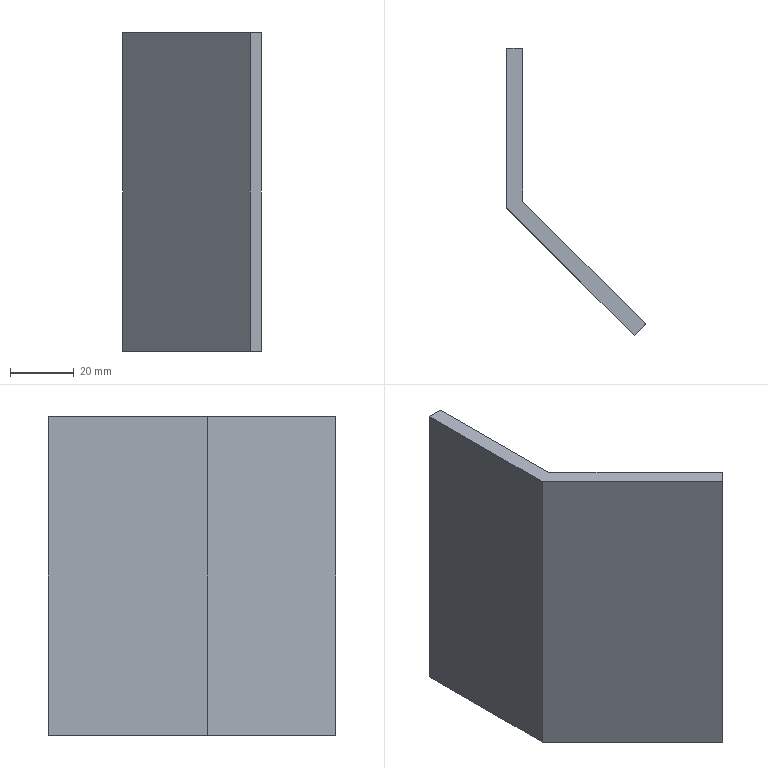Part | SolidWorks | features ICE 2, Extrusion 1 | 1 solid | 8 faces | box 43.536 x 90 x 100 mm | volume 52249 mm3 | plane 8
STEP:
#1=CARTESIAN_POINT('',(0.,0.,105.));
#2=VERTEX_POINT('',#1);
#3=CARTESIAN_POINT('',(0.,0.,5.));
#4=VERTEX_POINT('',#3);
#5=CARTESIAN_POINT('',(0.,0.,100.));
#6=DIRECTION('',(0.,0.,-1.));
#7=VECTOR('',#6,1000.);
#8=LINE('',#5,#7);
#9=EDGE_CURVE('',#2,#4,#8,.T.);
#10=ORIENTED_EDGE('',*,*,#9,.F.);
#11=CARTESIAN_POINT('',(5.,0.,105.));
#12=VERTEX_POINT('',#11);
#13=CARTESIAN_POINT('',(5.,0.,105.));
#14=DIRECTION('',(-1.,0.,0.));
#15=VECTOR('',#14,1000.);
#16=LINE('',#13,#15);
#17=EDGE_CURVE('',#12,#2,#16,.T.);
#18=ORIENTED_EDGE('',*,*,#17,.F.);
#19=CARTESIAN_POINT('',(5.,0.,5.));
#20=VERTEX_POINT('',#19);
#21=CARTESIAN_POINT('',(5.,0.,100.));
#22=DIRECTION('',(0.,0.,-1.));
#23=VECTOR('',#22,1000.);
#24=LINE('',#21,#23);
#25=EDGE_CURVE('',#12,#20,#24,.T.);
#26=ORIENTED_EDGE('',*,*,#25,.T.);
#27=CARTESIAN_POINT('',(0.,0.,5.));
#28=DIRECTION('',(1.,0.,0.));
#29=VECTOR('',#28,1000.);
#30=LINE('',#27,#29);
#31=EDGE_CURVE('',#4,#20,#30,.T.);
#32=ORIENTED_EDGE('',*,*,#31,.F.);
#33=EDGE_LOOP('',(#10,#18,#26,#32));
#34=FACE_OUTER_BOUND('',#33,.T.);
#35=CARTESIAN_POINT('',(0.,0.,100.));
#36=DIRECTION('',(0.,-1.,0.));
#37=DIRECTION('',(0.,0.,-1.));
#38=AXIS2_PLACEMENT_3D('',#35,#36,#37);
#39=PLANE('',#38);
#40=ADVANCED_FACE('',(#34),#39,.F.);
#41=CARTESIAN_POINT('',(0.,-50.,105.));
#42=VERTEX_POINT('',#41);
#43=CARTESIAN_POINT('',(0.,-50.,5.));
#44=VERTEX_POINT('',#43);
#45=CARTESIAN_POINT('',(0.,-50.,100.));
#46=DIRECTION('',(0.,0.,-1.));
#47=VECTOR('',#46,1000.);
#48=LINE('',#45,#47);
#49=EDGE_CURVE('',#42,#44,#48,.T.);
#50=ORIENTED_EDGE('',*,*,#49,.F.);
#51=CARTESIAN_POINT('',(0.,0.,105.));
#52=DIRECTION('',(0.,-1.,0.));
#53=VECTOR('',#52,1000.);
#54=LINE('',#51,#53);
#55=EDGE_CURVE('',#2,#42,#54,.T.);
#56=ORIENTED_EDGE('',*,*,#55,.F.);
#57=ORIENTED_EDGE('',*,*,#9,.T.);
#58=CARTESIAN_POINT('',(0.,0.,5.));
#59=DIRECTION('',(0.,-1.,0.));
#60=VECTOR('',#59,1000.);
#61=LINE('',#58,#60);
#62=EDGE_CURVE('',#4,#44,#61,.T.);
#63=ORIENTED_EDGE('',*,*,#62,.T.);
#64=EDGE_LOOP('',(#50,#56,#57,#63));
#65=FACE_OUTER_BOUND('',#64,.T.);
#66=CARTESIAN_POINT('',(0.,0.,100.));
#67=DIRECTION('',(1.,0.,0.));
#68=DIRECTION('',(0.,1.,0.));
#69=AXIS2_PLACEMENT_3D('',#66,#67,#68);
#70=PLANE('',#69);
#71=ADVANCED_FACE('',(#65),#70,.F.);
#72=CARTESIAN_POINT('',(40.,-90.,105.));
#73=VERTEX_POINT('',#72);
#74=CARTESIAN_POINT('',(40.,-90.,5.));
#75=VERTEX_POINT('',#74);
#76=CARTESIAN_POINT('',(40.,-90.,100.));
#77=DIRECTION('',(0.,0.,-1.));
#78=VECTOR('',#77,1000.);
#79=LINE('',#76,#78);
#80=EDGE_CURVE('',#73,#75,#79,.T.);
#81=ORIENTED_EDGE('',*,*,#80,.F.);
#82=CARTESIAN_POINT('',(0.,-50.,105.));
#83=DIRECTION('',(0.7071,-0.7071,0.));
#84=VECTOR('',#83,1000.);
#85=LINE('',#82,#84);
#86=EDGE_CURVE('',#42,#73,#85,.T.);
#87=ORIENTED_EDGE('',*,*,#86,.F.);
#88=ORIENTED_EDGE('',*,*,#49,.T.);
#89=CARTESIAN_POINT('',(0.,-50.,5.));
#90=DIRECTION('',(0.7071,-0.7071,0.));
#91=VECTOR('',#90,1000.);
#92=LINE('',#89,#91);
#93=EDGE_CURVE('',#44,#75,#92,.T.);
#94=ORIENTED_EDGE('',*,*,#93,.T.);
#95=EDGE_LOOP('',(#81,#87,#88,#94));
#96=FACE_OUTER_BOUND('',#95,.T.);
#97=CARTESIAN_POINT('',(0.,-50.,100.));
#98=DIRECTION('',(0.7071,0.7071,0.));
#99=DIRECTION('',(-0.7071,0.7071,0.));
#100=AXIS2_PLACEMENT_3D('',#97,#98,#99);
#101=PLANE('',#100);
#102=ADVANCED_FACE('',(#96),#101,.F.);
#103=CARTESIAN_POINT('',(43.536,-86.464,105.));
#104=VERTEX_POINT('',#103);
#105=CARTESIAN_POINT('',(43.536,-86.464,5.));
#106=VERTEX_POINT('',#105);
#107=CARTESIAN_POINT('',(43.536,-86.464,100.));
#108=DIRECTION('',(0.,0.,-1.));
#109=VECTOR('',#108,1000.);
#110=LINE('',#107,#109);
#111=EDGE_CURVE('',#104,#106,#110,.T.);
#112=ORIENTED_EDGE('',*,*,#111,.F.);
#113=CARTESIAN_POINT('',(40.,-90.,105.));
#114=DIRECTION('',(0.7071,0.7071,0.));
#115=VECTOR('',#114,1000.);
#116=LINE('',#113,#115);
#117=EDGE_CURVE('',#73,#104,#116,.T.);
#118=ORIENTED_EDGE('',*,*,#117,.F.);
#119=ORIENTED_EDGE('',*,*,#80,.T.);
#120=CARTESIAN_POINT('',(40.,-90.,5.));
#121=DIRECTION('',(0.7071,0.7071,0.));
#122=VECTOR('',#121,1000.);
#123=LINE('',#120,#122);
#124=EDGE_CURVE('',#75,#106,#123,.T.);
#125=ORIENTED_EDGE('',*,*,#124,.T.);
#126=EDGE_LOOP('',(#112,#118,#119,#125));
#127=FACE_OUTER_BOUND('',#126,.T.);
#128=CARTESIAN_POINT('',(40.,-90.,100.));
#129=DIRECTION('',(-0.7071,0.7071,0.));
#130=DIRECTION('',(-0.7071,-0.7071,0.));
#131=AXIS2_PLACEMENT_3D('',#128,#129,#130);
#132=PLANE('',#131);
#133=ADVANCED_FACE('',(#127),#132,.F.);
#134=CARTESIAN_POINT('',(5.,-47.929,105.));
#135=VERTEX_POINT('',#134);
#136=CARTESIAN_POINT('',(5.,-47.929,5.));
#137=VERTEX_POINT('',#136);
#138=CARTESIAN_POINT('',(5.,-47.929,100.));
#139=DIRECTION('',(0.,0.,-1.));
#140=VECTOR('',#139,1000.);
#141=LINE('',#138,#140);
#142=EDGE_CURVE('',#135,#137,#141,.T.);
#143=ORIENTED_EDGE('',*,*,#142,.F.);
#144=CARTESIAN_POINT('',(43.536,-86.464,105.));
#145=DIRECTION('',(-0.7071,0.7071,0.));
#146=VECTOR('',#145,1000.);
#147=LINE('',#144,#146);
#148=EDGE_CURVE('',#104,#135,#147,.T.);
#149=ORIENTED_EDGE('',*,*,#148,.F.);
#150=ORIENTED_EDGE('',*,*,#111,.T.);
#151=CARTESIAN_POINT('',(5.,-47.929,5.));
#152=DIRECTION('',(-0.7071,0.7071,0.));
#153=VECTOR('',#152,1000.);
#154=LINE('',#151,#153);
#155=EDGE_CURVE('',#106,#137,#154,.T.);
#156=ORIENTED_EDGE('',*,*,#155,.T.);
#157=EDGE_LOOP('',(#143,#149,#150,#156));
#158=FACE_OUTER_BOUND('',#157,.T.);
#159=CARTESIAN_POINT('',(5.,-47.929,100.));
#160=DIRECTION('',(-0.7071,-0.7071,0.));
#161=DIRECTION('',(0.7071,-0.7071,0.));
#162=AXIS2_PLACEMENT_3D('',#159,#160,#161);
#163=PLANE('',#162);
#164=ADVANCED_FACE('',(#158),#163,.F.);
#165=ORIENTED_EDGE('',*,*,#25,.F.);
#166=CARTESIAN_POINT('',(5.,-47.929,105.));
#167=DIRECTION('',(0.,1.,0.));
#168=VECTOR('',#167,1000.);
#169=LINE('',#166,#168);
#170=EDGE_CURVE('',#135,#12,#169,.T.);
#171=ORIENTED_EDGE('',*,*,#170,.F.);
#172=ORIENTED_EDGE('',*,*,#142,.T.);
#173=CARTESIAN_POINT('',(5.,0.,5.));
#174=DIRECTION('',(0.,1.,0.));
#175=VECTOR('',#174,1000.);
#176=LINE('',#173,#175);
#177=EDGE_CURVE('',#137,#20,#176,.T.);
#178=ORIENTED_EDGE('',*,*,#177,.T.);
#179=EDGE_LOOP('',(#165,#171,#172,#178));
#180=FACE_OUTER_BOUND('',#179,.T.);
#181=CARTESIAN_POINT('',(5.,0.,100.));
#182=DIRECTION('',(-1.,0.,0.));
#183=DIRECTION('',(0.,0.,1.));
#184=AXIS2_PLACEMENT_3D('',#181,#182,#183);
#185=PLANE('',#184);
#186=ADVANCED_FACE('',(#180),#185,.F.);
#187=ORIENTED_EDGE('',*,*,#62,.F.);
#188=ORIENTED_EDGE('',*,*,#31,.T.);
#189=ORIENTED_EDGE('',*,*,#177,.F.);
#190=ORIENTED_EDGE('',*,*,#155,.F.);
#191=ORIENTED_EDGE('',*,*,#124,.F.);
#192=ORIENTED_EDGE('',*,*,#93,.F.);
#193=EDGE_LOOP('',(#187,#188,#189,#190,#191,#192));
#194=FACE_OUTER_BOUND('',#193,.T.);
#195=CARTESIAN_POINT('',(0.,0.,5.));
#196=DIRECTION('',(0.,0.,1.));
#197=DIRECTION('',(1.,0.,0.));
#198=AXIS2_PLACEMENT_3D('',#195,#196,#197);
#199=PLANE('',#198);
#200=ADVANCED_FACE('',(#194),#199,.F.);
#201=ORIENTED_EDGE('',*,*,#55,.T.);
#202=ORIENTED_EDGE('',*,*,#86,.T.);
#203=ORIENTED_EDGE('',*,*,#117,.T.);
#204=ORIENTED_EDGE('',*,*,#148,.T.);
#205=ORIENTED_EDGE('',*,*,#170,.T.);
#206=ORIENTED_EDGE('',*,*,#17,.T.);
#207=EDGE_LOOP('',(#201,#202,#203,#204,#205,#206));
#208=FACE_OUTER_BOUND('',#207,.T.);
#209=CARTESIAN_POINT('',(0.,0.,105.));
#210=DIRECTION('',(0.,0.,-1.));
#211=DIRECTION('',(-1.,0.,0.));
#212=AXIS2_PLACEMENT_3D('',#209,#210,#211);
#213=PLANE('',#212);
#214=ADVANCED_FACE('',(#208),#213,.F.);
#215=CLOSED_SHELL('',(#40,#71,#102,#133,#164,#186,#200,#214));
#216=MANIFOLD_SOLID_BREP('',#215);
#217=CARTESIAN_POINT('',(0.,0.,0.));
#218=DIRECTION('',(0.,0.,1.));
#219=DIRECTION('',(1.,0.,0.));
#220=AXIS2_PLACEMENT_3D('',#217,#218,#219);
#221=(LENGTH_UNIT()NAMED_UNIT(*)SI_UNIT(.MILLI.,.METRE.));
#222=UNCERTAINTY_MEASURE_WITH_UNIT(LENGTH_MEASURE(0.00001),#221,'','');
#223=(NAMED_UNIT(*)PLANE_ANGLE_UNIT()SI_UNIT($,.RADIAN.));
#224=(NAMED_UNIT(*)SI_UNIT($,.STERADIAN.)SOLID_ANGLE_UNIT());
#225=(GEOMETRIC_REPRESENTATION_CONTEXT(3)GLOBAL_UNCERTAINTY_ASSIGNED_CONTEXT((#222))GLOBAL_UNIT_ASSIGNED_CONTEXT((#221,#223,#224))REPRESENTATION_CONTEXT('',''));
#226=ADVANCED_BREP_SHAPE_REPRESENTATION('',(#216,#220),#225);